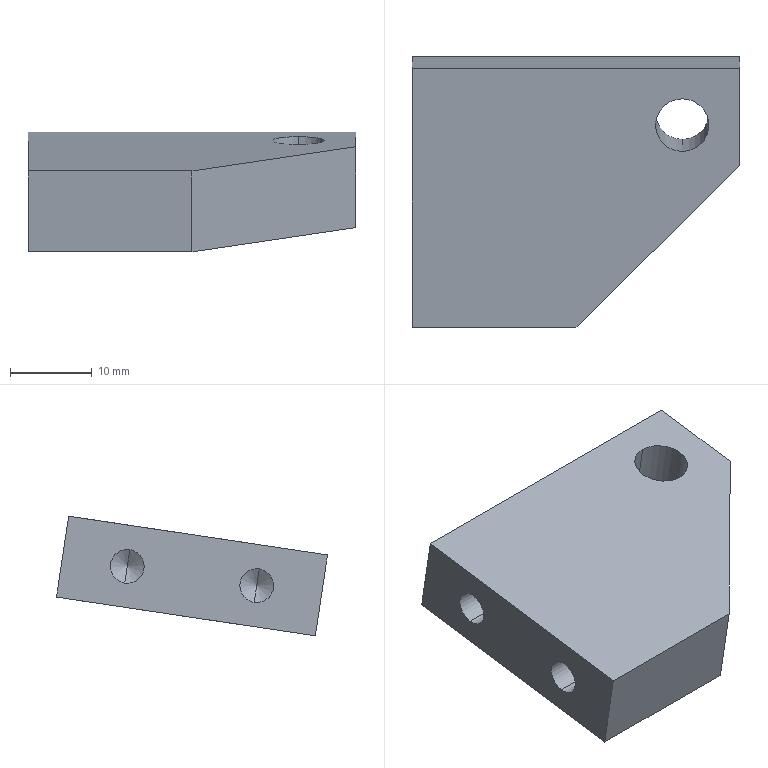Part | NX | features 实体1 2 | 1 solid | 17 faces | box 40 x 33.128 x 14.63 mm | volume 10189 mm3 | plane 7 | cylinder 6 | cone 4 | commonest cylinder face diameters 4.134 x4 6.5 x2
STEP:
#1=CARTESIAN_POINT('',(-80.041,146.744,-968.508));
#2=VERTEX_POINT('',#1);
#3=CARTESIAN_POINT('',(-80.041,140.316,-969.471));
#4=VERTEX_POINT('',#3);
#5=CARTESIAN_POINT('',(-80.041,143.53,-968.99));
#6=DIRECTION('',(0.,0.1481,-0.989));
#7=DIRECTION('',(0.,-0.989,-0.1481));
#8=AXIS2_PLACEMENT_3D('',#5,#6,#7);
#9=CIRCLE('',#8,3.25);
#10=EDGE_CURVE('',#2,#4,#9,.T.);
#11=ORIENTED_EDGE('',*,*,#10,.F.);
#12=CARTESIAN_POINT('',(-80.041,148.225,-978.398));
#13=VERTEX_POINT('',#12);
#14=CARTESIAN_POINT('',(-80.041,140.494,-926.782));
#15=DIRECTION('',(0.,0.1481,-0.989));
#16=VECTOR('',#15,1000.);
#17=LINE('',#14,#16);
#18=EDGE_CURVE('',#2,#13,#17,.T.);
#19=ORIENTED_EDGE('',*,*,#18,.T.);
#20=CARTESIAN_POINT('',(-80.041,141.797,-979.361));
#21=VERTEX_POINT('',#20);
#22=CARTESIAN_POINT('',(-80.041,145.011,-978.879));
#23=DIRECTION('',(0.,-0.1481,0.989));
#24=DIRECTION('',(0.,-0.989,-0.1481));
#25=AXIS2_PLACEMENT_3D('',#22,#23,#24);
#26=CIRCLE('',#25,3.25);
#27=EDGE_CURVE('',#21,#13,#26,.T.);
#28=ORIENTED_EDGE('',*,*,#27,.F.);
#29=CARTESIAN_POINT('',(-80.041,134.066,-927.745));
#30=DIRECTION('',(0.,0.1481,-0.989));
#31=VECTOR('',#30,1000.);
#32=LINE('',#29,#31);
#33=EDGE_CURVE('',#21,#4,#32,.F.);
#34=ORIENTED_EDGE('',*,*,#33,.T.);
#35=EDGE_LOOP('',(#11,#19,#28,#34));
#36=FACE_BOUND('',#35,.T.);
#37=CARTESIAN_POINT('',(-80.041,137.28,-927.263));
#38=DIRECTION('',(0.,0.1481,-0.989));
#39=DIRECTION('',(0.,0.989,0.1481));
#40=AXIS2_PLACEMENT_3D('',#37,#38,#39);
#41=CYLINDRICAL_SURFACE('',#40,3.25);
#42=ADVANCED_FACE('',(#36),#41,.F.);
#43=CARTESIAN_POINT('',(-103.041,142.976,-972.038));
#44=VERTEX_POINT('',#43);
#45=CARTESIAN_POINT('',(-103.041,143.588,-976.127));
#46=VERTEX_POINT('',#45);
#47=CARTESIAN_POINT('',(-103.041,143.282,-974.083));
#48=DIRECTION('',(-1.,0.,0.));
#49=DIRECTION('',(0.,0.1481,-0.989));
#50=AXIS2_PLACEMENT_3D('',#47,#48,#49);
#51=CIRCLE('',#50,2.067);
#52=EDGE_CURVE('',#44,#46,#51,.T.);
#53=ORIENTED_EDGE('',*,*,#52,.F.);
#54=CARTESIAN_POINT('',(-113.041,142.976,-972.038));
#55=VERTEX_POINT('',#54);
#56=CARTESIAN_POINT('',(-108.041,142.976,-972.038));
#57=DIRECTION('',(-1.,0.,0.));
#58=VECTOR('',#57,1000.);
#59=LINE('',#56,#58);
#60=EDGE_CURVE('',#44,#55,#59,.T.);
#61=ORIENTED_EDGE('',*,*,#60,.T.);
#62=CARTESIAN_POINT('',(-113.041,143.588,-976.127));
#63=VERTEX_POINT('',#62);
#64=CARTESIAN_POINT('',(-113.041,143.282,-974.083));
#65=DIRECTION('',(1.,0.,0.));
#66=DIRECTION('',(0.,0.1481,-0.989));
#67=AXIS2_PLACEMENT_3D('',#64,#65,#66);
#68=CIRCLE('',#67,2.067);
#69=EDGE_CURVE('',#63,#55,#68,.T.);
#70=ORIENTED_EDGE('',*,*,#69,.F.);
#71=CARTESIAN_POINT('',(-108.041,143.588,-976.127));
#72=DIRECTION('',(-1.,0.,0.));
#73=VECTOR('',#72,1000.);
#74=LINE('',#71,#73);
#75=EDGE_CURVE('',#63,#46,#74,.F.);
#76=ORIENTED_EDGE('',*,*,#75,.T.);
#77=EDGE_LOOP('',(#53,#61,#70,#76));
#78=FACE_BOUND('',#77,.T.);
#79=CARTESIAN_POINT('',(-108.041,143.282,-974.083));
#80=DIRECTION('',(-1.,0.,0.));
#81=DIRECTION('',(0.,-0.1481,0.989));
#82=AXIS2_PLACEMENT_3D('',#79,#80,#81);
#83=CYLINDRICAL_SURFACE('',#82,2.067);
#84=ADVANCED_FACE('',(#78),#83,.F.);
#85=CARTESIAN_POINT('',(-103.041,127.152,-974.409));
#86=VERTEX_POINT('',#85);
#87=CARTESIAN_POINT('',(-103.041,127.764,-978.497));
#88=VERTEX_POINT('',#87);
#89=CARTESIAN_POINT('',(-103.041,127.458,-976.453));
#90=DIRECTION('',(-1.,0.,0.));
#91=DIRECTION('',(0.,0.1481,-0.989));
#92=AXIS2_PLACEMENT_3D('',#89,#90,#91);
#93=CIRCLE('',#92,2.067);
#94=EDGE_CURVE('',#86,#88,#93,.T.);
#95=ORIENTED_EDGE('',*,*,#94,.F.);
#96=CARTESIAN_POINT('',(-113.041,127.152,-974.409));
#97=VERTEX_POINT('',#96);
#98=CARTESIAN_POINT('',(-108.041,127.152,-974.409));
#99=DIRECTION('',(-1.,0.,0.));
#100=VECTOR('',#99,1000.);
#101=LINE('',#98,#100);
#102=EDGE_CURVE('',#86,#97,#101,.T.);
#103=ORIENTED_EDGE('',*,*,#102,.T.);
#104=CARTESIAN_POINT('',(-113.041,127.764,-978.497));
#105=VERTEX_POINT('',#104);
#106=CARTESIAN_POINT('',(-113.041,127.458,-976.453));
#107=DIRECTION('',(1.,0.,0.));
#108=DIRECTION('',(0.,0.1481,-0.989));
#109=AXIS2_PLACEMENT_3D('',#106,#107,#108);
#110=CIRCLE('',#109,2.067);
#111=EDGE_CURVE('',#105,#97,#110,.T.);
#112=ORIENTED_EDGE('',*,*,#111,.F.);
#113=CARTESIAN_POINT('',(-108.041,127.764,-978.497));
#114=DIRECTION('',(-1.,0.,0.));
#115=VECTOR('',#114,1000.);
#116=LINE('',#113,#115);
#117=EDGE_CURVE('',#105,#88,#116,.F.);
#118=ORIENTED_EDGE('',*,*,#117,.T.);
#119=EDGE_LOOP('',(#95,#103,#112,#118));
#120=FACE_BOUND('',#119,.T.);
#121=CARTESIAN_POINT('',(-108.041,127.458,-976.453));
#122=DIRECTION('',(-1.,0.,0.));
#123=DIRECTION('',(0.,-0.1481,0.989));
#124=AXIS2_PLACEMENT_3D('',#121,#122,#123);
#125=CYLINDRICAL_SURFACE('',#124,2.067);
#126=ADVANCED_FACE('',(#120),#125,.F.);
#127=CARTESIAN_POINT('',(-101.799,143.282,-974.083));
#128=VERTEX_POINT('',#127);
#129=CARTESIAN_POINT('',(-103.041,143.588,-976.127));
#130=DIRECTION('',(-0.515,0.127,-0.8477));
#131=VECTOR('',#130,1000.);
#132=LINE('',#129,#131);
#133=EDGE_CURVE('',#46,#128,#132,.F.);
#134=ORIENTED_EDGE('',*,*,#133,.T.);
#135=CARTESIAN_POINT('',(-103.041,142.976,-972.038));
#136=DIRECTION('',(-0.515,-0.127,0.8477));
#137=VECTOR('',#136,1000.);
#138=LINE('',#135,#137);
#139=EDGE_CURVE('',#128,#44,#138,.T.);
#140=ORIENTED_EDGE('',*,*,#139,.T.);
#141=ORIENTED_EDGE('',*,*,#52,.T.);
#142=EDGE_LOOP('',(#134,#140,#141));
#143=FACE_BOUND('',#142,.T.);
#144=CARTESIAN_POINT('',(-103.041,143.282,-974.083));
#145=DIRECTION('',(-1.,0.,0.));
#146=DIRECTION('',(0.,-0.1481,0.989));
#147=AXIS2_PLACEMENT_3D('',#144,#145,#146);
#148=CONICAL_SURFACE('',#147,2.067,1.03);
#149=ADVANCED_FACE('',(#143),#148,.F.);
#150=CARTESIAN_POINT('',(-101.799,127.458,-976.453));
#151=VERTEX_POINT('',#150);
#152=CARTESIAN_POINT('',(-103.041,127.764,-978.497));
#153=DIRECTION('',(-0.515,0.127,-0.8477));
#154=VECTOR('',#153,1000.);
#155=LINE('',#152,#154);
#156=EDGE_CURVE('',#151,#88,#155,.T.);
#157=ORIENTED_EDGE('',*,*,#156,.F.);
#158=CARTESIAN_POINT('',(-103.041,127.152,-974.409));
#159=DIRECTION('',(-0.515,-0.127,0.8477));
#160=VECTOR('',#159,1000.);
#161=LINE('',#158,#160);
#162=EDGE_CURVE('',#86,#151,#161,.F.);
#163=ORIENTED_EDGE('',*,*,#162,.F.);
#164=ORIENTED_EDGE('',*,*,#94,.T.);
#165=EDGE_LOOP('',(#157,#163,#164));
#166=FACE_BOUND('',#165,.T.);
#167=CARTESIAN_POINT('',(-103.041,127.458,-976.453));
#168=DIRECTION('',(-1.,0.,0.));
#169=DIRECTION('',(0.,-0.1481,0.989));
#170=AXIS2_PLACEMENT_3D('',#167,#168,#169);
#171=CONICAL_SURFACE('',#170,2.067,1.03);
#172=ADVANCED_FACE('',(#166),#171,.F.);
#173=ORIENTED_EDGE('',*,*,#27,.T.);
#174=CARTESIAN_POINT('',(-80.041,145.011,-978.879));
#175=DIRECTION('',(0.,-0.1481,0.989));
#176=DIRECTION('',(0.,-0.989,-0.1481));
#177=AXIS2_PLACEMENT_3D('',#174,#175,#176);
#178=CIRCLE('',#177,3.25);
#179=EDGE_CURVE('',#13,#21,#178,.T.);
#180=ORIENTED_EDGE('',*,*,#179,.T.);
#181=EDGE_LOOP('',(#173,#180));
#182=FACE_BOUND('',#181,.T.);
#183=CARTESIAN_POINT('',(-113.041,151.934,-977.842));
#184=VERTEX_POINT('',#183);
#185=CARTESIAN_POINT('',(-73.041,151.934,-977.842));
#186=VERTEX_POINT('',#185);
#187=CARTESIAN_POINT('',(-93.041,151.934,-977.842));
#188=DIRECTION('',(1.,0.,0.));
#189=VECTOR('',#188,1000.);
#190=LINE('',#187,#189);
#191=EDGE_CURVE('',#184,#186,#190,.T.);
#192=ORIENTED_EDGE('',*,*,#191,.T.);
#193=CARTESIAN_POINT('',(-73.041,140.067,-979.62));
#194=VERTEX_POINT('',#193);
#195=CARTESIAN_POINT('',(-73.041,136.111,-980.213));
#196=DIRECTION('',(0.,-0.989,-0.1481));
#197=VECTOR('',#196,1000.);
#198=LINE('',#195,#197);
#199=EDGE_CURVE('',#186,#194,#198,.T.);
#200=ORIENTED_EDGE('',*,*,#199,.T.);
#201=CARTESIAN_POINT('',(-93.041,120.287,-982.583));
#202=VERTEX_POINT('',#201);
#203=CARTESIAN_POINT('',(-73.041,140.067,-979.62));
#204=DIRECTION('',(-0.7071,-0.6993,-0.1047));
#205=VECTOR('',#204,1000.);
#206=LINE('',#203,#205);
#207=EDGE_CURVE('',#194,#202,#206,.T.);
#208=ORIENTED_EDGE('',*,*,#207,.T.);
#209=CARTESIAN_POINT('',(-113.041,120.287,-982.583));
#210=VERTEX_POINT('',#209);
#211=CARTESIAN_POINT('',(-93.041,120.287,-982.583));
#212=DIRECTION('',(-1.,0.,0.));
#213=VECTOR('',#212,1000.);
#214=LINE('',#211,#213);
#215=EDGE_CURVE('',#202,#210,#214,.T.);
#216=ORIENTED_EDGE('',*,*,#215,.T.);
#217=CARTESIAN_POINT('',(-113.041,136.111,-980.213));
#218=DIRECTION('',(0.,0.989,0.1481));
#219=VECTOR('',#218,1000.);
#220=LINE('',#217,#219);
#221=EDGE_CURVE('',#210,#184,#220,.T.);
#222=ORIENTED_EDGE('',*,*,#221,.T.);
#223=EDGE_LOOP('',(#192,#200,#208,#216,#222));
#224=FACE_BOUND('',#223,.T.);
#225=CARTESIAN_POINT('',(-93.041,136.111,-980.213));
#226=DIRECTION('',(0.,0.1481,-0.989));
#227=DIRECTION('',(0.,0.989,0.1481));
#228=AXIS2_PLACEMENT_3D('',#225,#226,#227);
#229=PLANE('',#228);
#230=ADVANCED_FACE('',(#182,#224),#229,.T.);
#231=ORIENTED_EDGE('',*,*,#18,.F.);
#232=CARTESIAN_POINT('',(-80.041,143.53,-968.99));
#233=DIRECTION('',(0.,0.1481,-0.989));
#234=DIRECTION('',(0.,-0.989,-0.1481));
#235=AXIS2_PLACEMENT_3D('',#232,#233,#234);
#236=CIRCLE('',#235,3.25);
#237=EDGE_CURVE('',#4,#2,#236,.T.);
#238=ORIENTED_EDGE('',*,*,#237,.F.);
#239=ORIENTED_EDGE('',*,*,#33,.F.);
#240=ORIENTED_EDGE('',*,*,#179,.F.);
#241=EDGE_LOOP('',(#231,#238,#239,#240));
#242=FACE_BOUND('',#241,.T.);
#243=CARTESIAN_POINT('',(-80.041,137.28,-927.263));
#244=DIRECTION('',(0.,0.1481,-0.989));
#245=DIRECTION('',(0.,0.989,0.1481));
#246=AXIS2_PLACEMENT_3D('',#243,#244,#245);
#247=CYLINDRICAL_SURFACE('',#246,3.25);
#248=ADVANCED_FACE('',(#242),#247,.F.);
#249=CARTESIAN_POINT('',(-73.041,150.453,-967.953));
#250=VERTEX_POINT('',#249);
#251=CARTESIAN_POINT('',(-73.041,150.453,-967.953));
#252=DIRECTION('',(0.,-0.1481,0.989));
#253=VECTOR('',#252,1000.);
#254=LINE('',#251,#253);
#255=EDGE_CURVE('',#186,#250,#254,.T.);
#256=ORIENTED_EDGE('',*,*,#255,.T.);
#257=CARTESIAN_POINT('',(-73.041,138.585,-969.73));
#258=VERTEX_POINT('',#257);
#259=CARTESIAN_POINT('',(-73.041,118.806,-972.693));
#260=DIRECTION('',(0.,-0.989,-0.1481));
#261=VECTOR('',#260,1000.);
#262=LINE('',#259,#261);
#263=EDGE_CURVE('',#250,#258,#262,.T.);
#264=ORIENTED_EDGE('',*,*,#263,.T.);
#265=CARTESIAN_POINT('',(-73.041,138.585,-969.73));
#266=DIRECTION('',(0.,0.1481,-0.989));
#267=VECTOR('',#266,1000.);
#268=LINE('',#265,#267);
#269=EDGE_CURVE('',#258,#194,#268,.T.);
#270=ORIENTED_EDGE('',*,*,#269,.T.);
#271=ORIENTED_EDGE('',*,*,#199,.F.);
#272=EDGE_LOOP('',(#256,#264,#270,#271));
#273=FACE_BOUND('',#272,.T.);
#274=CARTESIAN_POINT('',(-73.041,118.806,-972.693));
#275=DIRECTION('',(1.,0.,0.));
#276=DIRECTION('',(0.,0.1481,-0.989));
#277=AXIS2_PLACEMENT_3D('',#274,#275,#276);
#278=PLANE('',#277);
#279=ADVANCED_FACE('',(#273),#278,.T.);
#280=CARTESIAN_POINT('',(-113.041,150.453,-967.953));
#281=VERTEX_POINT('',#280);
#282=CARTESIAN_POINT('',(-73.041,150.453,-967.953));
#283=DIRECTION('',(1.,0.,0.));
#284=VECTOR('',#283,1000.);
#285=LINE('',#282,#284);
#286=EDGE_CURVE('',#281,#250,#285,.T.);
#287=ORIENTED_EDGE('',*,*,#286,.T.);
#288=ORIENTED_EDGE('',*,*,#255,.F.);
#289=ORIENTED_EDGE('',*,*,#191,.F.);
#290=CARTESIAN_POINT('',(-113.041,150.453,-967.953));
#291=DIRECTION('',(0.,-0.1481,0.989));
#292=VECTOR('',#291,1000.);
#293=LINE('',#290,#292);
#294=EDGE_CURVE('',#184,#281,#293,.T.);
#295=ORIENTED_EDGE('',*,*,#294,.T.);
#296=EDGE_LOOP('',(#287,#288,#289,#295));
#297=FACE_BOUND('',#296,.T.);
#298=CARTESIAN_POINT('',(-73.041,150.453,-967.953));
#299=DIRECTION('',(0.,0.989,0.1481));
#300=DIRECTION('',(0.,-0.1481,0.989));
#301=AXIS2_PLACEMENT_3D('',#298,#299,#300);
#302=PLANE('',#301);
#303=ADVANCED_FACE('',(#297),#302,.T.);
#304=ORIENTED_EDGE('',*,*,#69,.T.);
#305=CARTESIAN_POINT('',(-113.041,143.282,-974.083));
#306=DIRECTION('',(1.,0.,0.));
#307=DIRECTION('',(0.,0.1481,-0.989));
#308=AXIS2_PLACEMENT_3D('',#305,#306,#307);
#309=CIRCLE('',#308,2.067);
#310=EDGE_CURVE('',#55,#63,#309,.T.);
#311=ORIENTED_EDGE('',*,*,#310,.T.);
#312=EDGE_LOOP('',(#304,#311));
#313=FACE_BOUND('',#312,.T.);
#314=ORIENTED_EDGE('',*,*,#111,.T.);
#315=CARTESIAN_POINT('',(-113.041,127.458,-976.453));
#316=DIRECTION('',(1.,0.,0.));
#317=DIRECTION('',(0.,0.1481,-0.989));
#318=AXIS2_PLACEMENT_3D('',#315,#316,#317);
#319=CIRCLE('',#318,2.067);
#320=EDGE_CURVE('',#97,#105,#319,.T.);
#321=ORIENTED_EDGE('',*,*,#320,.T.);
#322=EDGE_LOOP('',(#314,#321));
#323=FACE_BOUND('',#322,.T.);
#324=CARTESIAN_POINT('',(-113.041,118.806,-972.693));
#325=VERTEX_POINT('',#324);
#326=CARTESIAN_POINT('',(-113.041,150.453,-967.953));
#327=DIRECTION('',(0.,0.989,0.1481));
#328=VECTOR('',#327,1000.);
#329=LINE('',#326,#328);
#330=EDGE_CURVE('',#325,#281,#329,.T.);
#331=ORIENTED_EDGE('',*,*,#330,.T.);
#332=ORIENTED_EDGE('',*,*,#294,.F.);
#333=ORIENTED_EDGE('',*,*,#221,.F.);
#334=CARTESIAN_POINT('',(-113.041,118.806,-972.693));
#335=DIRECTION('',(0.,-0.1481,0.989));
#336=VECTOR('',#335,1000.);
#337=LINE('',#334,#336);
#338=EDGE_CURVE('',#210,#325,#337,.T.);
#339=ORIENTED_EDGE('',*,*,#338,.T.);
#340=EDGE_LOOP('',(#331,#332,#333,#339));
#341=FACE_BOUND('',#340,.T.);
#342=CARTESIAN_POINT('',(-113.041,150.453,-967.953));
#343=DIRECTION('',(-1.,0.,0.));
#344=DIRECTION('',(0.,-0.1481,0.989));
#345=AXIS2_PLACEMENT_3D('',#342,#343,#344);
#346=PLANE('',#345);
#347=ADVANCED_FACE('',(#313,#323,#341),#346,.T.);
#348=ORIENTED_EDGE('',*,*,#338,.F.);
#349=ORIENTED_EDGE('',*,*,#215,.F.);
#350=CARTESIAN_POINT('',(-93.041,118.806,-972.693));
#351=VERTEX_POINT('',#350);
#352=CARTESIAN_POINT('',(-93.041,118.806,-972.693));
#353=DIRECTION('',(0.,-0.1481,0.989));
#354=VECTOR('',#353,1000.);
#355=LINE('',#352,#354);
#356=EDGE_CURVE('',#202,#351,#355,.T.);
#357=ORIENTED_EDGE('',*,*,#356,.T.);
#358=CARTESIAN_POINT('',(-113.041,118.806,-972.693));
#359=DIRECTION('',(-1.,0.,0.));
#360=VECTOR('',#359,1000.);
#361=LINE('',#358,#360);
#362=EDGE_CURVE('',#351,#325,#361,.T.);
#363=ORIENTED_EDGE('',*,*,#362,.T.);
#364=EDGE_LOOP('',(#348,#349,#357,#363));
#365=FACE_BOUND('',#364,.T.);
#366=CARTESIAN_POINT('',(-113.041,118.806,-972.693));
#367=DIRECTION('',(0.,-0.989,-0.1481));
#368=DIRECTION('',(0.,0.1481,-0.989));
#369=AXIS2_PLACEMENT_3D('',#366,#367,#368);
#370=PLANE('',#369);
#371=ADVANCED_FACE('',(#365),#370,.T.);
#372=CARTESIAN_POINT('',(-83.041,128.696,-971.212));
#373=DIRECTION('',(-0.7071,-0.6993,-0.1047));
#374=VECTOR('',#373,1000.);
#375=LINE('',#372,#374);
#376=EDGE_CURVE('',#258,#351,#375,.T.);
#377=ORIENTED_EDGE('',*,*,#376,.T.);
#378=ORIENTED_EDGE('',*,*,#356,.F.);
#379=ORIENTED_EDGE('',*,*,#207,.F.);
#380=ORIENTED_EDGE('',*,*,#269,.F.);
#381=EDGE_LOOP('',(#377,#378,#379,#380));
#382=FACE_BOUND('',#381,.T.);
#383=CARTESIAN_POINT('',(-83.041,128.696,-971.212));
#384=DIRECTION('',(0.7071,-0.6993,-0.1047));
#385=DIRECTION('',(0.7071,0.6993,0.1047));
#386=AXIS2_PLACEMENT_3D('',#383,#384,#385);
#387=PLANE('',#386);
#388=ADVANCED_FACE('',(#382),#387,.T.);
#389=ORIENTED_EDGE('',*,*,#237,.T.);
#390=ORIENTED_EDGE('',*,*,#10,.T.);
#391=EDGE_LOOP('',(#389,#390));
#392=FACE_BOUND('',#391,.T.);
#393=ORIENTED_EDGE('',*,*,#263,.F.);
#394=ORIENTED_EDGE('',*,*,#286,.F.);
#395=ORIENTED_EDGE('',*,*,#330,.F.);
#396=ORIENTED_EDGE('',*,*,#362,.F.);
#397=ORIENTED_EDGE('',*,*,#376,.F.);
#398=EDGE_LOOP('',(#393,#394,#395,#396,#397));
#399=FACE_BOUND('',#398,.T.);
#400=CARTESIAN_POINT('',(-93.041,134.629,-970.323));
#401=DIRECTION('',(0.,0.1481,-0.989));
#402=DIRECTION('',(0.,0.989,0.1481));
#403=AXIS2_PLACEMENT_3D('',#400,#401,#402);
#404=PLANE('',#403);
#405=ADVANCED_FACE('',(#392,#399),#404,.F.);
#406=ORIENTED_EDGE('',*,*,#60,.F.);
#407=CARTESIAN_POINT('',(-103.041,143.282,-974.083));
#408=DIRECTION('',(-1.,0.,0.));
#409=DIRECTION('',(0.,0.1481,-0.989));
#410=AXIS2_PLACEMENT_3D('',#407,#408,#409);
#411=CIRCLE('',#410,2.067);
#412=EDGE_CURVE('',#46,#44,#411,.T.);
#413=ORIENTED_EDGE('',*,*,#412,.F.);
#414=ORIENTED_EDGE('',*,*,#75,.F.);
#415=ORIENTED_EDGE('',*,*,#310,.F.);
#416=EDGE_LOOP('',(#406,#413,#414,#415));
#417=FACE_BOUND('',#416,.T.);
#418=CARTESIAN_POINT('',(-108.041,143.282,-974.083));
#419=DIRECTION('',(-1.,0.,0.));
#420=DIRECTION('',(0.,-0.1481,0.989));
#421=AXIS2_PLACEMENT_3D('',#418,#419,#420);
#422=CYLINDRICAL_SURFACE('',#421,2.067);
#423=ADVANCED_FACE('',(#417),#422,.F.);
#424=ORIENTED_EDGE('',*,*,#102,.F.);
#425=CARTESIAN_POINT('',(-103.041,127.458,-976.453));
#426=DIRECTION('',(-1.,0.,0.));
#427=DIRECTION('',(0.,0.1481,-0.989));
#428=AXIS2_PLACEMENT_3D('',#425,#426,#427);
#429=CIRCLE('',#428,2.067);
#430=EDGE_CURVE('',#88,#86,#429,.T.);
#431=ORIENTED_EDGE('',*,*,#430,.F.);
#432=ORIENTED_EDGE('',*,*,#117,.F.);
#433=ORIENTED_EDGE('',*,*,#320,.F.);
#434=EDGE_LOOP('',(#424,#431,#432,#433));
#435=FACE_BOUND('',#434,.T.);
#436=CARTESIAN_POINT('',(-108.041,127.458,-976.453));
#437=DIRECTION('',(-1.,0.,0.));
#438=DIRECTION('',(0.,-0.1481,0.989));
#439=AXIS2_PLACEMENT_3D('',#436,#437,#438);
#440=CYLINDRICAL_SURFACE('',#439,2.067);
#441=ADVANCED_FACE('',(#435),#440,.F.);
#442=ORIENTED_EDGE('',*,*,#139,.F.);
#443=ORIENTED_EDGE('',*,*,#133,.F.);
#444=ORIENTED_EDGE('',*,*,#412,.T.);
#445=EDGE_LOOP('',(#442,#443,#444));
#446=FACE_BOUND('',#445,.T.);
#447=CARTESIAN_POINT('',(-103.041,143.282,-974.083));
#448=DIRECTION('',(-1.,0.,0.));
#449=DIRECTION('',(0.,-0.1481,0.989));
#450=AXIS2_PLACEMENT_3D('',#447,#448,#449);
#451=CONICAL_SURFACE('',#450,2.067,1.03);
#452=ADVANCED_FACE('',(#446),#451,.F.);
#453=ORIENTED_EDGE('',*,*,#162,.T.);
#454=ORIENTED_EDGE('',*,*,#156,.T.);
#455=ORIENTED_EDGE('',*,*,#430,.T.);
#456=EDGE_LOOP('',(#453,#454,#455));
#457=FACE_BOUND('',#456,.T.);
#458=CARTESIAN_POINT('',(-103.041,127.458,-976.453));
#459=DIRECTION('',(-1.,0.,0.));
#460=DIRECTION('',(0.,-0.1481,0.989));
#461=AXIS2_PLACEMENT_3D('',#458,#459,#460);
#462=CONICAL_SURFACE('',#461,2.067,1.03);
#463=ADVANCED_FACE('',(#457),#462,.F.);
#464=CLOSED_SHELL('',(#42,#84,#126,#149,#172,#230,#248,#279,#303,#347,#371,#388,#405,#423,#441,#452,#463));
#465=MANIFOLD_SOLID_BREP('',#464);
#466=(LENGTH_UNIT()NAMED_UNIT(*)SI_UNIT(.MILLI.,.METRE.));
#467=UNCERTAINTY_MEASURE_WITH_UNIT(LENGTH_MEASURE(0.00001),#466,'','');
#468=(NAMED_UNIT(*)PLANE_ANGLE_UNIT()SI_UNIT($,.RADIAN.));
#469=(NAMED_UNIT(*)SI_UNIT($,.STERADIAN.)SOLID_ANGLE_UNIT());
#470=(GEOMETRIC_REPRESENTATION_CONTEXT(3)GLOBAL_UNCERTAINTY_ASSIGNED_CONTEXT((#467))GLOBAL_UNIT_ASSIGNED_CONTEXT((#466,#468,#469))REPRESENTATION_CONTEXT('',''));
#471=ADVANCED_BREP_SHAPE_REPRESENTATION('',(#465),#470);